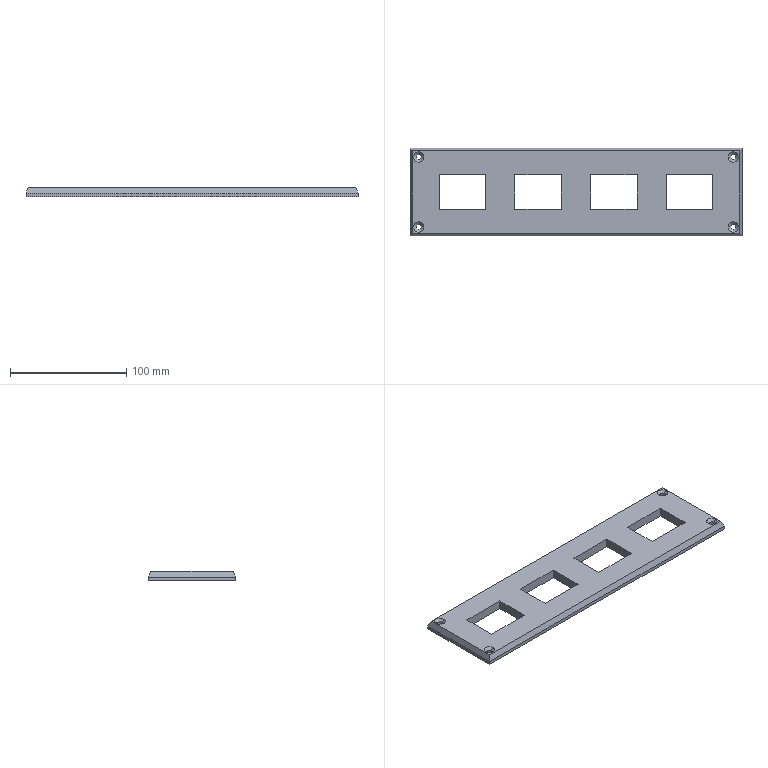Part | STEP file | DIP switch expansion board | 1 solid | 42 faces | box 285 x 75 x 8 mm | volume 128331 mm3 | plane 26 | cylinder 8 | cone 8 | commonest cylinder face diameters 4.5 x8